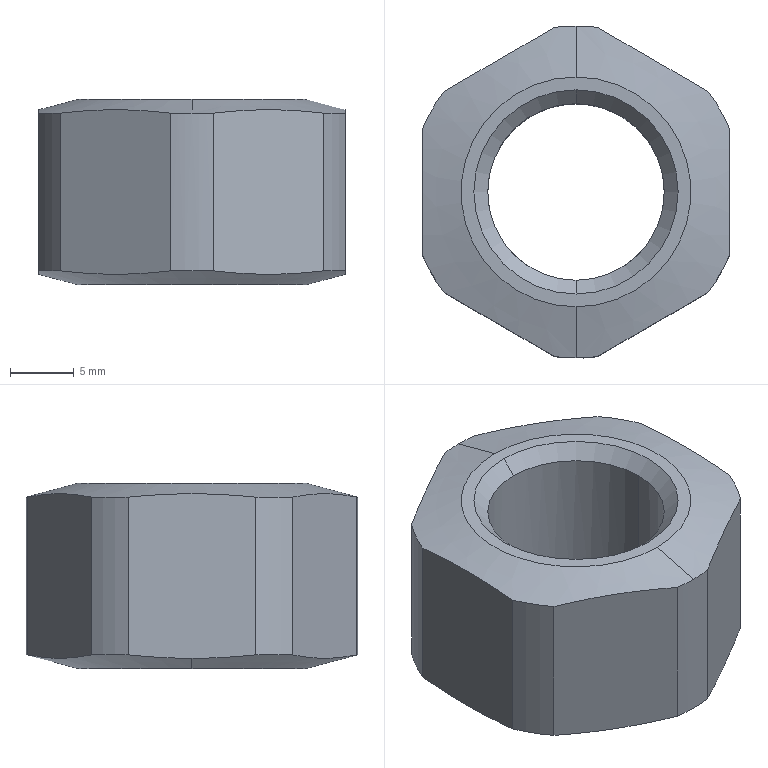Part | SolidWorks | features BaseBody 1 | 1 solid | 24 faces | box 24 x 26 x 14.5 mm | volume 4644 mm3 | cylinder 8 | cone 8 | plane 8 | commonest cylinder face diameters 26 x6 13.835 x2
STEP:
#1=CARTESIAN_POINT('',(-6.918,0.,-6.168));
#2=VERTEX_POINT('',#1);
#3=CARTESIAN_POINT('',(6.918,0.,-6.168));
#4=VERTEX_POINT('',#3);
#5=CARTESIAN_POINT('',(0.,0.,-6.168));
#6=DIRECTION('',(0.,0.,1.));
#7=DIRECTION('',(1.,0.,0.));
#8=AXIS2_PLACEMENT_3D('',#5,#6,#7);
#9=CIRCLE('',#8,6.918);
#10=EDGE_CURVE('',#2,#4,#9,.T.);
#11=ORIENTED_EDGE('',*,*,#10,.F.);
#12=CARTESIAN_POINT('',(-6.918,0.,6.168));
#13=VERTEX_POINT('',#12);
#14=CARTESIAN_POINT('',(-6.918,0.,-7.25));
#15=DIRECTION('',(0.,0.,1.));
#16=VECTOR('',#15,1000.);
#17=LINE('',#14,#16);
#18=EDGE_CURVE('',#2,#13,#17,.T.);
#19=ORIENTED_EDGE('',*,*,#18,.T.);
#20=CARTESIAN_POINT('',(0.,-6.918,6.168));
#21=VERTEX_POINT('',#20);
#22=CARTESIAN_POINT('',(0.,0.,6.168));
#23=DIRECTION('',(0.,0.,-1.));
#24=DIRECTION('',(1.,0.,0.));
#25=AXIS2_PLACEMENT_3D('',#22,#23,#24);
#26=CIRCLE('',#25,6.918);
#27=EDGE_CURVE('',#21,#13,#26,.T.);
#28=ORIENTED_EDGE('',*,*,#27,.F.);
#29=CARTESIAN_POINT('',(6.918,0.,6.168));
#30=VERTEX_POINT('',#29);
#31=CARTESIAN_POINT('',(0.,0.,6.168));
#32=DIRECTION('',(0.,0.,-1.));
#33=DIRECTION('',(1.,0.,0.));
#34=AXIS2_PLACEMENT_3D('',#31,#32,#33);
#35=CIRCLE('',#34,6.918);
#36=EDGE_CURVE('',#30,#21,#35,.T.);
#37=ORIENTED_EDGE('',*,*,#36,.F.);
#38=CARTESIAN_POINT('',(6.918,0.,-7.25));
#39=DIRECTION('',(0.,0.,1.));
#40=VECTOR('',#39,1000.);
#41=LINE('',#38,#40);
#42=EDGE_CURVE('',#4,#30,#41,.T.);
#43=ORIENTED_EDGE('',*,*,#42,.F.);
#44=EDGE_LOOP('',(#11,#19,#28,#37,#43));
#45=FACE_OUTER_BOUND('',#44,.T.);
#46=CARTESIAN_POINT('',(0.,0.,-7.25));
#47=DIRECTION('',(0.,0.,1.));
#48=DIRECTION('',(1.,0.,0.));
#49=AXIS2_PLACEMENT_3D('',#46,#47,#48);
#50=CYLINDRICAL_SURFACE('',#49,6.918);
#51=ADVANCED_FACE('',(#45),#50,.F.);
#52=ORIENTED_EDGE('',*,*,#27,.T.);
#53=CARTESIAN_POINT('',(0.,6.918,6.168));
#54=VERTEX_POINT('',#53);
#55=CARTESIAN_POINT('',(0.,0.,6.168));
#56=DIRECTION('',(0.,0.,-1.));
#57=DIRECTION('',(1.,0.,0.));
#58=AXIS2_PLACEMENT_3D('',#55,#56,#57);
#59=CIRCLE('',#58,6.918);
#60=EDGE_CURVE('',#13,#54,#59,.T.);
#61=ORIENTED_EDGE('',*,*,#60,.T.);
#62=CARTESIAN_POINT('',(0.,8.,7.25));
#63=VERTEX_POINT('',#62);
#64=CARTESIAN_POINT('',(0.,8.,7.25));
#65=DIRECTION('',(0.,0.7071,0.7071));
#66=VECTOR('',#65,1000.);
#67=LINE('',#64,#66);
#68=EDGE_CURVE('',#54,#63,#67,.T.);
#69=ORIENTED_EDGE('',*,*,#68,.T.);
#70=CARTESIAN_POINT('',(0.,-8.,7.25));
#71=VERTEX_POINT('',#70);
#72=CARTESIAN_POINT('',(0.,0.,7.25));
#73=DIRECTION('',(0.,0.,-1.));
#74=DIRECTION('',(0.,-1.,0.));
#75=AXIS2_PLACEMENT_3D('',#72,#73,#74);
#76=CIRCLE('',#75,8.);
#77=EDGE_CURVE('',#71,#63,#76,.T.);
#78=ORIENTED_EDGE('',*,*,#77,.F.);
#79=CARTESIAN_POINT('',(0.,-8.,7.25));
#80=DIRECTION('',(0.,-0.7071,0.7071));
#81=VECTOR('',#80,1000.);
#82=LINE('',#79,#81);
#83=EDGE_CURVE('',#21,#71,#82,.T.);
#84=ORIENTED_EDGE('',*,*,#83,.F.);
#85=EDGE_LOOP('',(#52,#61,#69,#78,#84));
#86=FACE_OUTER_BOUND('',#85,.T.);
#87=CARTESIAN_POINT('',(0.,0.,7.25));
#88=DIRECTION('',(0.,0.,1.));
#89=DIRECTION('',(0.,-1.,0.));
#90=AXIS2_PLACEMENT_3D('',#87,#88,#89);
#91=CONICAL_SURFACE('',#90,8.,0.7854);
#92=ADVANCED_FACE('',(#86),#91,.F.);
#93=ORIENTED_EDGE('',*,*,#10,.T.);
#94=CARTESIAN_POINT('',(8.,0.,-7.25));
#95=VERTEX_POINT('',#94);
#96=CARTESIAN_POINT('',(8.,0.,-7.25));
#97=DIRECTION('',(0.7071,0.,-0.7071));
#98=VECTOR('',#97,1000.);
#99=LINE('',#96,#98);
#100=EDGE_CURVE('',#4,#95,#99,.T.);
#101=ORIENTED_EDGE('',*,*,#100,.T.);
#102=CARTESIAN_POINT('',(-8.,0.,-7.25));
#103=VERTEX_POINT('',#102);
#104=CARTESIAN_POINT('',(0.,0.,-7.25));
#105=DIRECTION('',(0.,0.,1.));
#106=DIRECTION('',(-1.,0.,0.));
#107=AXIS2_PLACEMENT_3D('',#104,#105,#106);
#108=CIRCLE('',#107,8.);
#109=EDGE_CURVE('',#103,#95,#108,.T.);
#110=ORIENTED_EDGE('',*,*,#109,.F.);
#111=CARTESIAN_POINT('',(-8.,0.,-7.25));
#112=DIRECTION('',(-0.7071,0.,-0.7071));
#113=VECTOR('',#112,1000.);
#114=LINE('',#111,#113);
#115=EDGE_CURVE('',#2,#103,#114,.T.);
#116=ORIENTED_EDGE('',*,*,#115,.F.);
#117=EDGE_LOOP('',(#93,#101,#110,#116));
#118=FACE_OUTER_BOUND('',#117,.T.);
#119=CARTESIAN_POINT('',(0.,0.,-7.25));
#120=DIRECTION('',(0.,0.,-1.));
#121=DIRECTION('',(-1.,0.,0.));
#122=AXIS2_PLACEMENT_3D('',#119,#120,#121);
#123=CONICAL_SURFACE('',#122,8.,0.7854);
#124=ADVANCED_FACE('',(#118),#123,.F.);
#125=CARTESIAN_POINT('',(0.,9.,7.25));
#126=VERTEX_POINT('',#125);
#127=CARTESIAN_POINT('',(0.,-9.,7.25));
#128=VERTEX_POINT('',#127);
#129=CARTESIAN_POINT('',(0.,0.,7.25));
#130=DIRECTION('',(0.,0.,-1.));
#131=DIRECTION('',(0.,1.,0.));
#132=AXIS2_PLACEMENT_3D('',#129,#130,#131);
#133=CIRCLE('',#132,9.);
#134=EDGE_CURVE('',#126,#128,#133,.T.);
#135=ORIENTED_EDGE('',*,*,#134,.T.);
#136=CARTESIAN_POINT('',(0.,-13.,6.178));
#137=VERTEX_POINT('',#136);
#138=CARTESIAN_POINT('',(0.,-13.,6.178));
#139=DIRECTION('',(0.,-0.9659,-0.2588));
#140=VECTOR('',#139,1000.);
#141=LINE('',#138,#140);
#142=EDGE_CURVE('',#128,#137,#141,.T.);
#143=ORIENTED_EDGE('',*,*,#142,.T.);
#144=CARTESIAN_POINT('',(1.67,-12.892,6.178));
#145=VERTEX_POINT('',#144);
#146=CARTESIAN_POINT('',(0.,0.,6.178));
#147=DIRECTION('',(0.,0.,1.));
#148=DIRECTION('',(-1.,0.,0.));
#149=AXIS2_PLACEMENT_3D('',#146,#147,#148);
#150=CIRCLE('',#149,13.);
#151=EDGE_CURVE('',#137,#145,#150,.T.);
#152=ORIENTED_EDGE('',*,*,#151,.T.);
#153=CARTESIAN_POINT('',(10.33,-7.892,6.178));
#154=VERTEX_POINT('',#153);
#155=CARTESIAN_POINT('',(1.67,-12.892,6.178));
#156=CARTESIAN_POINT('',(3.113,-12.059,6.35));
#157=CARTESIAN_POINT('',(6.,-10.392,6.542));
#158=CARTESIAN_POINT('',(8.887,-8.726,6.35));
#159=CARTESIAN_POINT('',(10.33,-7.892,6.178));
#160=B_SPLINE_CURVE_WITH_KNOTS('',3,(#155,#156,#157,#158,#159),.UNSPECIFIED.,.F.,.F.,(4,1,4),(0.,0.005,0.01),.UNSPECIFIED.);
#161=EDGE_CURVE('',#145,#154,#160,.T.);
#162=ORIENTED_EDGE('',*,*,#161,.T.);
#163=CARTESIAN_POINT('',(12.,-5.,6.178));
#164=VERTEX_POINT('',#163);
#165=CARTESIAN_POINT('',(0.,0.,6.178));
#166=DIRECTION('',(0.,0.,1.));
#167=DIRECTION('',(-1.,0.,0.));
#168=AXIS2_PLACEMENT_3D('',#165,#166,#167);
#169=CIRCLE('',#168,13.);
#170=EDGE_CURVE('',#154,#164,#169,.T.);
#171=ORIENTED_EDGE('',*,*,#170,.T.);
#172=CARTESIAN_POINT('',(12.,5.,6.178));
#173=VERTEX_POINT('',#172);
#174=CARTESIAN_POINT('',(12.,-5.,6.178));
#175=CARTESIAN_POINT('',(12.,-3.333,6.35));
#176=CARTESIAN_POINT('',(12.,0.,6.542));
#177=CARTESIAN_POINT('',(12.,3.333,6.35));
#178=CARTESIAN_POINT('',(12.,5.,6.178));
#179=B_SPLINE_CURVE_WITH_KNOTS('',3,(#174,#175,#176,#177,#178),.UNSPECIFIED.,.F.,.F.,(4,1,4),(0.,0.005,0.01),.UNSPECIFIED.);
#180=EDGE_CURVE('',#164,#173,#179,.T.);
#181=ORIENTED_EDGE('',*,*,#180,.T.);
#182=CARTESIAN_POINT('',(10.33,7.892,6.178));
#183=VERTEX_POINT('',#182);
#184=CARTESIAN_POINT('',(0.,0.,6.178));
#185=DIRECTION('',(0.,0.,1.));
#186=DIRECTION('',(-1.,0.,0.));
#187=AXIS2_PLACEMENT_3D('',#184,#185,#186);
#188=CIRCLE('',#187,13.);
#189=EDGE_CURVE('',#173,#183,#188,.T.);
#190=ORIENTED_EDGE('',*,*,#189,.T.);
#191=CARTESIAN_POINT('',(1.67,12.892,6.178));
#192=VERTEX_POINT('',#191);
#193=CARTESIAN_POINT('',(10.33,7.892,6.178));
#194=CARTESIAN_POINT('',(8.887,8.726,6.35));
#195=CARTESIAN_POINT('',(6.,10.392,6.542));
#196=CARTESIAN_POINT('',(3.113,12.059,6.35));
#197=CARTESIAN_POINT('',(1.67,12.892,6.178));
#198=B_SPLINE_CURVE_WITH_KNOTS('',3,(#193,#194,#195,#196,#197),.UNSPECIFIED.,.F.,.F.,(4,1,4),(0.,0.005,0.01),.UNSPECIFIED.);
#199=EDGE_CURVE('',#183,#192,#198,.T.);
#200=ORIENTED_EDGE('',*,*,#199,.T.);
#201=CARTESIAN_POINT('',(0.,13.,6.178));
#202=VERTEX_POINT('',#201);
#203=CARTESIAN_POINT('',(0.,0.,6.178));
#204=DIRECTION('',(0.,0.,1.));
#205=DIRECTION('',(-1.,0.,0.));
#206=AXIS2_PLACEMENT_3D('',#203,#204,#205);
#207=CIRCLE('',#206,13.);
#208=EDGE_CURVE('',#192,#202,#207,.T.);
#209=ORIENTED_EDGE('',*,*,#208,.T.);
#210=CARTESIAN_POINT('',(0.,13.,6.178));
#211=DIRECTION('',(0.,0.9659,-0.2588));
#212=VECTOR('',#211,1000.);
#213=LINE('',#210,#212);
#214=EDGE_CURVE('',#126,#202,#213,.T.);
#215=ORIENTED_EDGE('',*,*,#214,.F.);
#216=EDGE_LOOP('',(#135,#143,#152,#162,#171,#181,#190,#200,#209,#215));
#217=FACE_OUTER_BOUND('',#216,.T.);
#218=CARTESIAN_POINT('',(0.,0.,6.178));
#219=DIRECTION('',(0.,0.,-1.));
#220=DIRECTION('',(0.,1.,0.));
#221=AXIS2_PLACEMENT_3D('',#218,#219,#220);
#222=CONICAL_SURFACE('',#221,13.,1.309);
#223=ADVANCED_FACE('',(#217),#222,.T.);
#224=CARTESIAN_POINT('',(9.,0.,-7.25));
#225=VERTEX_POINT('',#224);
#226=CARTESIAN_POINT('',(-9.,0.,-7.25));
#227=VERTEX_POINT('',#226);
#228=CARTESIAN_POINT('',(0.,0.,-7.25));
#229=DIRECTION('',(0.,0.,1.));
#230=DIRECTION('',(1.,0.,0.));
#231=AXIS2_PLACEMENT_3D('',#228,#229,#230);
#232=CIRCLE('',#231,9.);
#233=EDGE_CURVE('',#225,#227,#232,.T.);
#234=ORIENTED_EDGE('',*,*,#233,.T.);
#235=CARTESIAN_POINT('',(-12.,0.,-6.446));
#236=VERTEX_POINT('',#235);
#237=CARTESIAN_POINT('',(-13.,0.,-6.178));
#238=DIRECTION('',(-0.9659,0.,0.2588));
#239=VECTOR('',#238,1000.);
#240=LINE('',#237,#239);
#241=EDGE_CURVE('',#227,#236,#240,.T.);
#242=ORIENTED_EDGE('',*,*,#241,.T.);
#243=CARTESIAN_POINT('',(-12.,5.,-6.178));
#244=VERTEX_POINT('',#243);
#245=CARTESIAN_POINT('',(-12.,0.,-6.446));
#246=CARTESIAN_POINT('',(-12.,1.667,-6.446));
#247=CARTESIAN_POINT('',(-12.,3.333,-6.35));
#248=CARTESIAN_POINT('',(-12.,5.,-6.178));
#249=B_SPLINE_CURVE_WITH_KNOTS('',3,(#245,#246,#247,#248),.UNSPECIFIED.,.F.,.F.,(4,4),(0.005,0.01),.UNSPECIFIED.);
#250=EDGE_CURVE('',#236,#244,#249,.T.);
#251=ORIENTED_EDGE('',*,*,#250,.T.);
#252=CARTESIAN_POINT('',(-10.33,7.892,-6.178));
#253=VERTEX_POINT('',#252);
#254=CARTESIAN_POINT('',(0.,0.,-6.178));
#255=DIRECTION('',(0.,0.,-1.));
#256=DIRECTION('',(1.,0.,0.));
#257=AXIS2_PLACEMENT_3D('',#254,#255,#256);
#258=CIRCLE('',#257,13.);
#259=EDGE_CURVE('',#244,#253,#258,.T.);
#260=ORIENTED_EDGE('',*,*,#259,.T.);
#261=CARTESIAN_POINT('',(-1.67,12.892,-6.178));
#262=VERTEX_POINT('',#261);
#263=CARTESIAN_POINT('',(-10.33,7.892,-6.178));
#264=CARTESIAN_POINT('',(-8.887,8.726,-6.35));
#265=CARTESIAN_POINT('',(-6.,10.392,-6.542));
#266=CARTESIAN_POINT('',(-3.113,12.059,-6.35));
#267=CARTESIAN_POINT('',(-1.67,12.892,-6.178));
#268=B_SPLINE_CURVE_WITH_KNOTS('',3,(#263,#264,#265,#266,#267),.UNSPECIFIED.,.F.,.F.,(4,1,4),(0.,0.005,0.01),.UNSPECIFIED.);
#269=EDGE_CURVE('',#253,#262,#268,.T.);
#270=ORIENTED_EDGE('',*,*,#269,.T.);
#271=CARTESIAN_POINT('',(1.67,12.892,-6.178));
#272=VERTEX_POINT('',#271);
#273=CARTESIAN_POINT('',(0.,0.,-6.178));
#274=DIRECTION('',(0.,0.,-1.));
#275=DIRECTION('',(1.,0.,0.));
#276=AXIS2_PLACEMENT_3D('',#273,#274,#275);
#277=CIRCLE('',#276,13.);
#278=EDGE_CURVE('',#262,#272,#277,.T.);
#279=ORIENTED_EDGE('',*,*,#278,.T.);
#280=CARTESIAN_POINT('',(10.33,7.892,-6.178));
#281=VERTEX_POINT('',#280);
#282=CARTESIAN_POINT('',(1.67,12.892,-6.178));
#283=CARTESIAN_POINT('',(3.113,12.059,-6.35));
#284=CARTESIAN_POINT('',(6.,10.392,-6.542));
#285=CARTESIAN_POINT('',(8.887,8.726,-6.35));
#286=CARTESIAN_POINT('',(10.33,7.892,-6.178));
#287=B_SPLINE_CURVE_WITH_KNOTS('',3,(#282,#283,#284,#285,#286),.UNSPECIFIED.,.F.,.F.,(4,1,4),(0.,0.005,0.01),.UNSPECIFIED.);
#288=EDGE_CURVE('',#272,#281,#287,.T.);
#289=ORIENTED_EDGE('',*,*,#288,.T.);
#290=CARTESIAN_POINT('',(12.,5.,-6.178));
#291=VERTEX_POINT('',#290);
#292=CARTESIAN_POINT('',(0.,0.,-6.178));
#293=DIRECTION('',(0.,0.,-1.));
#294=DIRECTION('',(1.,0.,0.));
#295=AXIS2_PLACEMENT_3D('',#292,#293,#294);
#296=CIRCLE('',#295,13.);
#297=EDGE_CURVE('',#281,#291,#296,.T.);
#298=ORIENTED_EDGE('',*,*,#297,.T.);
#299=CARTESIAN_POINT('',(12.,0.,-6.446));
#300=VERTEX_POINT('',#299);
#301=CARTESIAN_POINT('',(12.,5.,-6.178));
#302=CARTESIAN_POINT('',(12.,3.333,-6.35));
#303=CARTESIAN_POINT('',(12.,1.667,-6.446));
#304=CARTESIAN_POINT('',(12.,0.,-6.446));
#305=B_SPLINE_CURVE_WITH_KNOTS('',3,(#301,#302,#303,#304),.UNSPECIFIED.,.F.,.F.,(4,4),(0.,0.005),.UNSPECIFIED.);
#306=EDGE_CURVE('',#291,#300,#305,.T.);
#307=ORIENTED_EDGE('',*,*,#306,.T.);
#308=CARTESIAN_POINT('',(13.,0.,-6.178));
#309=DIRECTION('',(0.9659,0.,0.2588));
#310=VECTOR('',#309,1000.);
#311=LINE('',#308,#310);
#312=EDGE_CURVE('',#225,#300,#311,.T.);
#313=ORIENTED_EDGE('',*,*,#312,.F.);
#314=EDGE_LOOP('',(#234,#242,#251,#260,#270,#279,#289,#298,#307,#313));
#315=FACE_OUTER_BOUND('',#314,.T.);
#316=CARTESIAN_POINT('',(0.,0.,-6.178));
#317=DIRECTION('',(0.,0.,1.));
#318=DIRECTION('',(1.,0.,0.));
#319=AXIS2_PLACEMENT_3D('',#316,#317,#318);
#320=CONICAL_SURFACE('',#319,13.,1.309);
#321=ADVANCED_FACE('',(#315),#320,.T.);
#322=ORIENTED_EDGE('',*,*,#18,.F.);
#323=CARTESIAN_POINT('',(0.,0.,-6.168));
#324=DIRECTION('',(0.,0.,1.));
#325=DIRECTION('',(1.,0.,0.));
#326=AXIS2_PLACEMENT_3D('',#323,#324,#325);
#327=CIRCLE('',#326,6.918);
#328=EDGE_CURVE('',#4,#2,#327,.T.);
#329=ORIENTED_EDGE('',*,*,#328,.F.);
#330=ORIENTED_EDGE('',*,*,#42,.T.);
#331=CARTESIAN_POINT('',(0.,0.,6.168));
#332=DIRECTION('',(0.,0.,-1.));
#333=DIRECTION('',(1.,0.,0.));
#334=AXIS2_PLACEMENT_3D('',#331,#332,#333);
#335=CIRCLE('',#334,6.918);
#336=EDGE_CURVE('',#54,#30,#335,.T.);
#337=ORIENTED_EDGE('',*,*,#336,.F.);
#338=ORIENTED_EDGE('',*,*,#60,.F.);
#339=EDGE_LOOP('',(#322,#329,#330,#337,#338));
#340=FACE_OUTER_BOUND('',#339,.T.);
#341=CARTESIAN_POINT('',(0.,0.,-7.25));
#342=DIRECTION('',(0.,0.,1.));
#343=DIRECTION('',(1.,0.,0.));
#344=AXIS2_PLACEMENT_3D('',#341,#342,#343);
#345=CYLINDRICAL_SURFACE('',#344,6.918);
#346=ADVANCED_FACE('',(#340),#345,.F.);
#347=ORIENTED_EDGE('',*,*,#68,.F.);
#348=ORIENTED_EDGE('',*,*,#336,.T.);
#349=ORIENTED_EDGE('',*,*,#36,.T.);
#350=ORIENTED_EDGE('',*,*,#83,.T.);
#351=CARTESIAN_POINT('',(0.,0.,7.25));
#352=DIRECTION('',(0.,0.,-1.));
#353=DIRECTION('',(0.,-1.,0.));
#354=AXIS2_PLACEMENT_3D('',#351,#352,#353);
#355=CIRCLE('',#354,8.);
#356=EDGE_CURVE('',#63,#71,#355,.T.);
#357=ORIENTED_EDGE('',*,*,#356,.F.);
#358=EDGE_LOOP('',(#347,#348,#349,#350,#357));
#359=FACE_OUTER_BOUND('',#358,.T.);
#360=CARTESIAN_POINT('',(0.,0.,7.25));
#361=DIRECTION('',(0.,0.,1.));
#362=DIRECTION('',(0.,-1.,0.));
#363=AXIS2_PLACEMENT_3D('',#360,#361,#362);
#364=CONICAL_SURFACE('',#363,8.,0.7854);
#365=ADVANCED_FACE('',(#359),#364,.F.);
#366=ORIENTED_EDGE('',*,*,#100,.F.);
#367=ORIENTED_EDGE('',*,*,#328,.T.);
#368=ORIENTED_EDGE('',*,*,#115,.T.);
#369=CARTESIAN_POINT('',(0.,0.,-7.25));
#370=DIRECTION('',(0.,0.,1.));
#371=DIRECTION('',(-1.,0.,0.));
#372=AXIS2_PLACEMENT_3D('',#369,#370,#371);
#373=CIRCLE('',#372,8.);
#374=EDGE_CURVE('',#95,#103,#373,.T.);
#375=ORIENTED_EDGE('',*,*,#374,.F.);
#376=EDGE_LOOP('',(#366,#367,#368,#375));
#377=FACE_OUTER_BOUND('',#376,.T.);
#378=CARTESIAN_POINT('',(0.,0.,-7.25));
#379=DIRECTION('',(0.,0.,-1.));
#380=DIRECTION('',(-1.,0.,0.));
#381=AXIS2_PLACEMENT_3D('',#378,#379,#380);
#382=CONICAL_SURFACE('',#381,8.,0.7854);
#383=ADVANCED_FACE('',(#377),#382,.F.);
#384=ORIENTED_EDGE('',*,*,#77,.T.);
#385=ORIENTED_EDGE('',*,*,#356,.T.);
#386=EDGE_LOOP('',(#384,#385));
#387=FACE_BOUND('',#386,.T.);
#388=ORIENTED_EDGE('',*,*,#134,.F.);
#389=CARTESIAN_POINT('',(0.,0.,7.25));
#390=DIRECTION('',(0.,0.,-1.));
#391=DIRECTION('',(0.,1.,0.));
#392=AXIS2_PLACEMENT_3D('',#389,#390,#391);
#393=CIRCLE('',#392,9.);
#394=EDGE_CURVE('',#128,#126,#393,.T.);
#395=ORIENTED_EDGE('',*,*,#394,.F.);
#396=EDGE_LOOP('',(#388,#395));
#397=FACE_OUTER_BOUND('',#396,.T.);
#398=CARTESIAN_POINT('',(0.,0.,7.25));
#399=DIRECTION('',(0.,0.,-1.));
#400=DIRECTION('',(-1.,0.,0.));
#401=AXIS2_PLACEMENT_3D('',#398,#399,#400);
#402=PLANE('',#401);
#403=ADVANCED_FACE('',(#387,#397),#402,.F.);
#404=ORIENTED_EDGE('',*,*,#233,.F.);
#405=CARTESIAN_POINT('',(0.,0.,-7.25));
#406=DIRECTION('',(0.,0.,1.));
#407=DIRECTION('',(1.,0.,0.));
#408=AXIS2_PLACEMENT_3D('',#405,#406,#407);
#409=CIRCLE('',#408,9.);
#410=EDGE_CURVE('',#227,#225,#409,.T.);
#411=ORIENTED_EDGE('',*,*,#410,.F.);
#412=EDGE_LOOP('',(#404,#411));
#413=FACE_OUTER_BOUND('',#412,.T.);
#414=ORIENTED_EDGE('',*,*,#109,.T.);
#415=ORIENTED_EDGE('',*,*,#374,.T.);
#416=EDGE_LOOP('',(#414,#415));
#417=FACE_BOUND('',#416,.T.);
#418=CARTESIAN_POINT('',(0.,9.,-7.25));
#419=DIRECTION('',(0.,0.,1.));
#420=DIRECTION('',(1.,0.,0.));
#421=AXIS2_PLACEMENT_3D('',#418,#419,#420);
#422=PLANE('',#421);
#423=ADVANCED_FACE('',(#413,#417),#422,.F.);
#424=ORIENTED_EDGE('',*,*,#142,.F.);
#425=ORIENTED_EDGE('',*,*,#394,.T.);
#426=ORIENTED_EDGE('',*,*,#214,.T.);
#427=CARTESIAN_POINT('',(-1.67,12.892,6.178));
#428=VERTEX_POINT('',#427);
#429=CARTESIAN_POINT('',(0.,0.,6.178));
#430=DIRECTION('',(0.,0.,1.));
#431=DIRECTION('',(-1.,0.,0.));
#432=AXIS2_PLACEMENT_3D('',#429,#430,#431);
#433=CIRCLE('',#432,13.);
#434=EDGE_CURVE('',#202,#428,#433,.T.);
#435=ORIENTED_EDGE('',*,*,#434,.T.);
#436=CARTESIAN_POINT('',(-10.33,7.892,6.178));
#437=VERTEX_POINT('',#436);
#438=CARTESIAN_POINT('',(-1.67,12.892,6.178));
#439=CARTESIAN_POINT('',(-3.113,12.059,6.35));
#440=CARTESIAN_POINT('',(-6.,10.392,6.542));
#441=CARTESIAN_POINT('',(-8.887,8.726,6.35));
#442=CARTESIAN_POINT('',(-10.33,7.892,6.178));
#443=B_SPLINE_CURVE_WITH_KNOTS('',3,(#438,#439,#440,#441,#442),.UNSPECIFIED.,.F.,.F.,(4,1,4),(0.,0.005,0.01),.UNSPECIFIED.);
#444=EDGE_CURVE('',#428,#437,#443,.T.);
#445=ORIENTED_EDGE('',*,*,#444,.T.);
#446=CARTESIAN_POINT('',(-12.,5.,6.178));
#447=VERTEX_POINT('',#446);
#448=CARTESIAN_POINT('',(0.,0.,6.178));
#449=DIRECTION('',(0.,0.,1.));
#450=DIRECTION('',(-1.,0.,0.));
#451=AXIS2_PLACEMENT_3D('',#448,#449,#450);
#452=CIRCLE('',#451,13.);
#453=EDGE_CURVE('',#437,#447,#452,.T.);
#454=ORIENTED_EDGE('',*,*,#453,.T.);
#455=CARTESIAN_POINT('',(-12.,-5.,6.178));
#456=VERTEX_POINT('',#455);
#457=CARTESIAN_POINT('',(-12.,5.,6.178));
#458=CARTESIAN_POINT('',(-12.,3.333,6.35));
#459=CARTESIAN_POINT('',(-12.,0.,6.542));
#460=CARTESIAN_POINT('',(-12.,-3.333,6.35));
#461=CARTESIAN_POINT('',(-12.,-5.,6.178));
#462=B_SPLINE_CURVE_WITH_KNOTS('',3,(#457,#458,#459,#460,#461),.UNSPECIFIED.,.F.,.F.,(4,1,4),(0.,0.005,0.01),.UNSPECIFIED.);
#463=EDGE_CURVE('',#447,#456,#462,.T.);
#464=ORIENTED_EDGE('',*,*,#463,.T.);
#465=CARTESIAN_POINT('',(-10.33,-7.892,6.178));
#466=VERTEX_POINT('',#465);
#467=CARTESIAN_POINT('',(0.,0.,6.178));
#468=DIRECTION('',(0.,0.,1.));
#469=DIRECTION('',(-1.,0.,0.));
#470=AXIS2_PLACEMENT_3D('',#467,#468,#469);
#471=CIRCLE('',#470,13.);
#472=EDGE_CURVE('',#456,#466,#471,.T.);
#473=ORIENTED_EDGE('',*,*,#472,.T.);
#474=CARTESIAN_POINT('',(-1.67,-12.892,6.178));
#475=VERTEX_POINT('',#474);
#476=CARTESIAN_POINT('',(-10.33,-7.892,6.178));
#477=CARTESIAN_POINT('',(-8.887,-8.726,6.35));
#478=CARTESIAN_POINT('',(-6.,-10.392,6.542));
#479=CARTESIAN_POINT('',(-3.113,-12.059,6.35));
#480=CARTESIAN_POINT('',(-1.67,-12.892,6.178));
#481=B_SPLINE_CURVE_WITH_KNOTS('',3,(#476,#477,#478,#479,#480),.UNSPECIFIED.,.F.,.F.,(4,1,4),(0.,0.005,0.01),.UNSPECIFIED.);
#482=EDGE_CURVE('',#466,#475,#481,.T.);
#483=ORIENTED_EDGE('',*,*,#482,.T.);
#484=CARTESIAN_POINT('',(0.,0.,6.178));
#485=DIRECTION('',(0.,0.,1.));
#486=DIRECTION('',(-1.,0.,0.));
#487=AXIS2_PLACEMENT_3D('',#484,#485,#486);
#488=CIRCLE('',#487,13.);
#489=EDGE_CURVE('',#475,#137,#488,.T.);
#490=ORIENTED_EDGE('',*,*,#489,.T.);
#491=EDGE_LOOP('',(#424,#425,#426,#435,#445,#454,#464,#473,#483,#490));
#492=FACE_OUTER_BOUND('',#491,.T.);
#493=CARTESIAN_POINT('',(0.,0.,6.178));
#494=DIRECTION('',(0.,0.,-1.));
#495=DIRECTION('',(0.,1.,0.));
#496=AXIS2_PLACEMENT_3D('',#493,#494,#495);
#497=CONICAL_SURFACE('',#496,13.,1.309);
#498=ADVANCED_FACE('',(#492),#497,.T.);
#499=ORIENTED_EDGE('',*,*,#241,.F.);
#500=ORIENTED_EDGE('',*,*,#410,.T.);
#501=ORIENTED_EDGE('',*,*,#312,.T.);
#502=CARTESIAN_POINT('',(12.,-5.,-6.178));
#503=VERTEX_POINT('',#502);
#504=CARTESIAN_POINT('',(12.,0.,-6.446));
#505=CARTESIAN_POINT('',(12.,-1.667,-6.446));
#506=CARTESIAN_POINT('',(12.,-3.333,-6.35));
#507=CARTESIAN_POINT('',(12.,-5.,-6.178));
#508=B_SPLINE_CURVE_WITH_KNOTS('',3,(#504,#505,#506,#507),.UNSPECIFIED.,.F.,.F.,(4,4),(0.005,0.01),.UNSPECIFIED.);
#509=EDGE_CURVE('',#300,#503,#508,.T.);
#510=ORIENTED_EDGE('',*,*,#509,.T.);
#511=CARTESIAN_POINT('',(10.33,-7.892,-6.178));
#512=VERTEX_POINT('',#511);
#513=CARTESIAN_POINT('',(0.,0.,-6.178));
#514=DIRECTION('',(0.,0.,-1.));
#515=DIRECTION('',(1.,0.,0.));
#516=AXIS2_PLACEMENT_3D('',#513,#514,#515);
#517=CIRCLE('',#516,13.);
#518=EDGE_CURVE('',#503,#512,#517,.T.);
#519=ORIENTED_EDGE('',*,*,#518,.T.);
#520=CARTESIAN_POINT('',(1.67,-12.892,-6.178));
#521=VERTEX_POINT('',#520);
#522=CARTESIAN_POINT('',(10.33,-7.892,-6.178));
#523=CARTESIAN_POINT('',(8.887,-8.726,-6.35));
#524=CARTESIAN_POINT('',(6.,-10.392,-6.542));
#525=CARTESIAN_POINT('',(3.113,-12.059,-6.35));
#526=CARTESIAN_POINT('',(1.67,-12.892,-6.178));
#527=B_SPLINE_CURVE_WITH_KNOTS('',3,(#522,#523,#524,#525,#526),.UNSPECIFIED.,.F.,.F.,(4,1,4),(0.,0.005,0.01),.UNSPECIFIED.);
#528=EDGE_CURVE('',#512,#521,#527,.T.);
#529=ORIENTED_EDGE('',*,*,#528,.T.);
#530=CARTESIAN_POINT('',(-1.67,-12.892,-6.178));
#531=VERTEX_POINT('',#530);
#532=CARTESIAN_POINT('',(0.,0.,-6.178));
#533=DIRECTION('',(0.,0.,-1.));
#534=DIRECTION('',(1.,0.,0.));
#535=AXIS2_PLACEMENT_3D('',#532,#533,#534);
#536=CIRCLE('',#535,13.);
#537=EDGE_CURVE('',#521,#531,#536,.T.);
#538=ORIENTED_EDGE('',*,*,#537,.T.);
#539=CARTESIAN_POINT('',(-10.33,-7.892,-6.178));
#540=VERTEX_POINT('',#539);
#541=CARTESIAN_POINT('',(-1.67,-12.892,-6.178));
#542=CARTESIAN_POINT('',(-3.113,-12.059,-6.35));
#543=CARTESIAN_POINT('',(-6.,-10.392,-6.542));
#544=CARTESIAN_POINT('',(-8.887,-8.726,-6.35));
#545=CARTESIAN_POINT('',(-10.33,-7.892,-6.178));
#546=B_SPLINE_CURVE_WITH_KNOTS('',3,(#541,#542,#543,#544,#545),.UNSPECIFIED.,.F.,.F.,(4,1,4),(0.,0.005,0.01),.UNSPECIFIED.);
#547=EDGE_CURVE('',#531,#540,#546,.T.);
#548=ORIENTED_EDGE('',*,*,#547,.T.);
#549=CARTESIAN_POINT('',(-12.,-5.,-6.178));
#550=VERTEX_POINT('',#549);
#551=CARTESIAN_POINT('',(0.,0.,-6.178));
#552=DIRECTION('',(0.,0.,-1.));
#553=DIRECTION('',(1.,0.,0.));
#554=AXIS2_PLACEMENT_3D('',#551,#552,#553);
#555=CIRCLE('',#554,13.);
#556=EDGE_CURVE('',#540,#550,#555,.T.);
#557=ORIENTED_EDGE('',*,*,#556,.T.);
#558=CARTESIAN_POINT('',(-12.,-5.,-6.178));
#559=CARTESIAN_POINT('',(-12.,-3.333,-6.35));
#560=CARTESIAN_POINT('',(-12.,-1.667,-6.446));
#561=CARTESIAN_POINT('',(-12.,0.,-6.446));
#562=B_SPLINE_CURVE_WITH_KNOTS('',3,(#558,#559,#560,#561),.UNSPECIFIED.,.F.,.F.,(4,4),(0.,0.005),.UNSPECIFIED.);
#563=EDGE_CURVE('',#550,#236,#562,.T.);
#564=ORIENTED_EDGE('',*,*,#563,.T.);
#565=EDGE_LOOP('',(#499,#500,#501,#510,#519,#529,#538,#548,#557,#564));
#566=FACE_OUTER_BOUND('',#565,.T.);
#567=CARTESIAN_POINT('',(0.,0.,-6.178));
#568=DIRECTION('',(0.,0.,1.));
#569=DIRECTION('',(1.,0.,0.));
#570=AXIS2_PLACEMENT_3D('',#567,#568,#569);
#571=CONICAL_SURFACE('',#570,13.,1.309);
#572=ADVANCED_FACE('',(#566),#571,.T.);
#573=CARTESIAN_POINT('',(1.67,12.892,7.25));
#574=DIRECTION('',(0.,0.,-1.));
#575=VECTOR('',#574,1000.);
#576=LINE('',#573,#575);
#577=EDGE_CURVE('',#192,#272,#576,.T.);
#578=ORIENTED_EDGE('',*,*,#577,.F.);
#579=ORIENTED_EDGE('',*,*,#199,.F.);
#580=CARTESIAN_POINT('',(10.33,7.892,7.25));
#581=DIRECTION('',(0.,0.,1.));
#582=VECTOR('',#581,1000.);
#583=LINE('',#580,#582);
#584=EDGE_CURVE('',#281,#183,#583,.T.);
#585=ORIENTED_EDGE('',*,*,#584,.F.);
#586=ORIENTED_EDGE('',*,*,#288,.F.);
#587=EDGE_LOOP('',(#578,#579,#585,#586));
#588=FACE_OUTER_BOUND('',#587,.T.);
#589=CARTESIAN_POINT('',(12.,6.928,7.25));
#590=DIRECTION('',(-0.5,-0.866,0.));
#591=DIRECTION('',(0.866,-0.5,0.));
#592=AXIS2_PLACEMENT_3D('',#589,#590,#591);
#593=PLANE('',#592);
#594=ADVANCED_FACE('',(#588),#593,.F.);
#595=ORIENTED_EDGE('',*,*,#584,.T.);
#596=ORIENTED_EDGE('',*,*,#189,.F.);
#597=CARTESIAN_POINT('',(12.,5.,7.25));
#598=DIRECTION('',(0.,0.,-1.));
#599=VECTOR('',#598,1000.);
#600=LINE('',#597,#599);
#601=EDGE_CURVE('',#173,#291,#600,.T.);
#602=ORIENTED_EDGE('',*,*,#601,.T.);
#603=ORIENTED_EDGE('',*,*,#297,.F.);
#604=EDGE_LOOP('',(#595,#596,#602,#603));
#605=FACE_OUTER_BOUND('',#604,.T.);
#606=CARTESIAN_POINT('',(0.,0.,7.25));
#607=DIRECTION('',(0.,0.,1.));
#608=DIRECTION('',(1.,0.,0.));
#609=AXIS2_PLACEMENT_3D('',#606,#607,#608);
#610=CYLINDRICAL_SURFACE('',#609,13.);
#611=ADVANCED_FACE('',(#605),#610,.T.);
#612=ORIENTED_EDGE('',*,*,#601,.F.);
#613=ORIENTED_EDGE('',*,*,#180,.F.);
#614=CARTESIAN_POINT('',(12.,-5.,7.25));
#615=DIRECTION('',(0.,0.,1.));
#616=VECTOR('',#615,1000.);
#617=LINE('',#614,#616);
#618=EDGE_CURVE('',#503,#164,#617,.T.);
#619=ORIENTED_EDGE('',*,*,#618,.F.);
#620=ORIENTED_EDGE('',*,*,#509,.F.);
#621=ORIENTED_EDGE('',*,*,#306,.F.);
#622=EDGE_LOOP('',(#612,#613,#619,#620,#621));
#623=FACE_OUTER_BOUND('',#622,.T.);
#624=CARTESIAN_POINT('',(12.,-6.928,7.25));
#625=DIRECTION('',(-1.,0.,0.));
#626=DIRECTION('',(0.,0.,1.));
#627=AXIS2_PLACEMENT_3D('',#624,#625,#626);
#628=PLANE('',#627);
#629=ADVANCED_FACE('',(#623),#628,.F.);
#630=ORIENTED_EDGE('',*,*,#618,.T.);
#631=ORIENTED_EDGE('',*,*,#170,.F.);
#632=CARTESIAN_POINT('',(10.33,-7.892,7.25));
#633=DIRECTION('',(0.,0.,-1.));
#634=VECTOR('',#633,1000.);
#635=LINE('',#632,#634);
#636=EDGE_CURVE('',#154,#512,#635,.T.);
#637=ORIENTED_EDGE('',*,*,#636,.T.);
#638=ORIENTED_EDGE('',*,*,#518,.F.);
#639=EDGE_LOOP('',(#630,#631,#637,#638));
#640=FACE_OUTER_BOUND('',#639,.T.);
#641=CARTESIAN_POINT('',(0.,0.,7.25));
#642=DIRECTION('',(0.,0.,1.));
#643=DIRECTION('',(1.,0.,0.));
#644=AXIS2_PLACEMENT_3D('',#641,#642,#643);
#645=CYLINDRICAL_SURFACE('',#644,13.);
#646=ADVANCED_FACE('',(#640),#645,.T.);
#647=ORIENTED_EDGE('',*,*,#636,.F.);
#648=ORIENTED_EDGE('',*,*,#161,.F.);
#649=CARTESIAN_POINT('',(1.67,-12.892,7.25));
#650=DIRECTION('',(0.,0.,1.));
#651=VECTOR('',#650,1000.);
#652=LINE('',#649,#651);
#653=EDGE_CURVE('',#521,#145,#652,.T.);
#654=ORIENTED_EDGE('',*,*,#653,.F.);
#655=ORIENTED_EDGE('',*,*,#528,.F.);
#656=EDGE_LOOP('',(#647,#648,#654,#655));
#657=FACE_OUTER_BOUND('',#656,.T.);
#658=CARTESIAN_POINT('',(0.,-13.856,7.25));
#659=DIRECTION('',(-0.5,0.866,0.));
#660=DIRECTION('',(-0.866,-0.5,0.));
#661=AXIS2_PLACEMENT_3D('',#658,#659,#660);
#662=PLANE('',#661);
#663=ADVANCED_FACE('',(#657),#662,.F.);
#664=ORIENTED_EDGE('',*,*,#653,.T.);
#665=ORIENTED_EDGE('',*,*,#151,.F.);
#666=ORIENTED_EDGE('',*,*,#489,.F.);
#667=CARTESIAN_POINT('',(-1.67,-12.892,7.25));
#668=DIRECTION('',(0.,0.,-1.));
#669=VECTOR('',#668,1000.);
#670=LINE('',#667,#669);
#671=EDGE_CURVE('',#475,#531,#670,.T.);
#672=ORIENTED_EDGE('',*,*,#671,.T.);
#673=ORIENTED_EDGE('',*,*,#537,.F.);
#674=EDGE_LOOP('',(#664,#665,#666,#672,#673));
#675=FACE_OUTER_BOUND('',#674,.T.);
#676=CARTESIAN_POINT('',(0.,0.,7.25));
#677=DIRECTION('',(0.,0.,1.));
#678=DIRECTION('',(1.,0.,0.));
#679=AXIS2_PLACEMENT_3D('',#676,#677,#678);
#680=CYLINDRICAL_SURFACE('',#679,13.);
#681=ADVANCED_FACE('',(#675),#680,.T.);
#682=ORIENTED_EDGE('',*,*,#671,.F.);
#683=ORIENTED_EDGE('',*,*,#482,.F.);
#684=CARTESIAN_POINT('',(-10.33,-7.892,7.25));
#685=DIRECTION('',(0.,0.,1.));
#686=VECTOR('',#685,1000.);
#687=LINE('',#684,#686);
#688=EDGE_CURVE('',#540,#466,#687,.T.);
#689=ORIENTED_EDGE('',*,*,#688,.F.);
#690=ORIENTED_EDGE('',*,*,#547,.F.);
#691=EDGE_LOOP('',(#682,#683,#689,#690));
#692=FACE_OUTER_BOUND('',#691,.T.);
#693=CARTESIAN_POINT('',(-12.,-6.928,7.25));
#694=DIRECTION('',(0.5,0.866,0.));
#695=DIRECTION('',(-0.866,0.5,0.));
#696=AXIS2_PLACEMENT_3D('',#693,#694,#695);
#697=PLANE('',#696);
#698=ADVANCED_FACE('',(#692),#697,.F.);
#699=ORIENTED_EDGE('',*,*,#688,.T.);
#700=ORIENTED_EDGE('',*,*,#472,.F.);
#701=CARTESIAN_POINT('',(-12.,-5.,7.25));
#702=DIRECTION('',(0.,0.,-1.));
#703=VECTOR('',#702,1000.);
#704=LINE('',#701,#703);
#705=EDGE_CURVE('',#456,#550,#704,.T.);
#706=ORIENTED_EDGE('',*,*,#705,.T.);
#707=ORIENTED_EDGE('',*,*,#556,.F.);
#708=EDGE_LOOP('',(#699,#700,#706,#707));
#709=FACE_OUTER_BOUND('',#708,.T.);
#710=CARTESIAN_POINT('',(0.,0.,7.25));
#711=DIRECTION('',(0.,0.,1.));
#712=DIRECTION('',(1.,0.,0.));
#713=AXIS2_PLACEMENT_3D('',#710,#711,#712);
#714=CYLINDRICAL_SURFACE('',#713,13.);
#715=ADVANCED_FACE('',(#709),#714,.T.);
#716=ORIENTED_EDGE('',*,*,#705,.F.);
#717=ORIENTED_EDGE('',*,*,#463,.F.);
#718=CARTESIAN_POINT('',(-12.,5.,7.25));
#719=DIRECTION('',(0.,0.,1.));
#720=VECTOR('',#719,1000.);
#721=LINE('',#718,#720);
#722=EDGE_CURVE('',#244,#447,#721,.T.);
#723=ORIENTED_EDGE('',*,*,#722,.F.);
#724=ORIENTED_EDGE('',*,*,#250,.F.);
#725=ORIENTED_EDGE('',*,*,#563,.F.);
#726=EDGE_LOOP('',(#716,#717,#723,#724,#725));
#727=FACE_OUTER_BOUND('',#726,.T.);
#728=CARTESIAN_POINT('',(-12.,6.928,7.25));
#729=DIRECTION('',(1.,0.,0.));
#730=DIRECTION('',(0.,0.,-1.));
#731=AXIS2_PLACEMENT_3D('',#728,#729,#730);
#732=PLANE('',#731);
#733=ADVANCED_FACE('',(#727),#732,.F.);
#734=ORIENTED_EDGE('',*,*,#722,.T.);
#735=ORIENTED_EDGE('',*,*,#453,.F.);
#736=CARTESIAN_POINT('',(-10.33,7.892,7.25));
#737=DIRECTION('',(0.,0.,-1.));
#738=VECTOR('',#737,1000.);
#739=LINE('',#736,#738);
#740=EDGE_CURVE('',#437,#253,#739,.T.);
#741=ORIENTED_EDGE('',*,*,#740,.T.);
#742=ORIENTED_EDGE('',*,*,#259,.F.);
#743=EDGE_LOOP('',(#734,#735,#741,#742));
#744=FACE_OUTER_BOUND('',#743,.T.);
#745=CARTESIAN_POINT('',(0.,0.,7.25));
#746=DIRECTION('',(0.,0.,1.));
#747=DIRECTION('',(1.,0.,0.));
#748=AXIS2_PLACEMENT_3D('',#745,#746,#747);
#749=CYLINDRICAL_SURFACE('',#748,13.);
#750=ADVANCED_FACE('',(#744),#749,.T.);
#751=ORIENTED_EDGE('',*,*,#740,.F.);
#752=ORIENTED_EDGE('',*,*,#444,.F.);
#753=CARTESIAN_POINT('',(-1.67,12.892,7.25));
#754=DIRECTION('',(0.,0.,1.));
#755=VECTOR('',#754,1000.);
#756=LINE('',#753,#755);
#757=EDGE_CURVE('',#262,#428,#756,.T.);
#758=ORIENTED_EDGE('',*,*,#757,.F.);
#759=ORIENTED_EDGE('',*,*,#269,.F.);
#760=EDGE_LOOP('',(#751,#752,#758,#759));
#761=FACE_OUTER_BOUND('',#760,.T.);
#762=CARTESIAN_POINT('',(0.,13.856,7.25));
#763=DIRECTION('',(0.5,-0.866,0.));
#764=DIRECTION('',(0.866,0.5,0.));
#765=AXIS2_PLACEMENT_3D('',#762,#763,#764);
#766=PLANE('',#765);
#767=ADVANCED_FACE('',(#761),#766,.F.);
#768=ORIENTED_EDGE('',*,*,#757,.T.);
#769=ORIENTED_EDGE('',*,*,#434,.F.);
#770=ORIENTED_EDGE('',*,*,#208,.F.);
#771=ORIENTED_EDGE('',*,*,#577,.T.);
#772=ORIENTED_EDGE('',*,*,#278,.F.);
#773=EDGE_LOOP('',(#768,#769,#770,#771,#772));
#774=FACE_OUTER_BOUND('',#773,.T.);
#775=CARTESIAN_POINT('',(0.,0.,7.25));
#776=DIRECTION('',(0.,0.,1.));
#777=DIRECTION('',(1.,0.,0.));
#778=AXIS2_PLACEMENT_3D('',#775,#776,#777);
#779=CYLINDRICAL_SURFACE('',#778,13.);
#780=ADVANCED_FACE('',(#774),#779,.T.);
#781=CLOSED_SHELL('',(#51,#92,#124,#223,#321,#346,#365,#383,#403,#423,#498,#572,#594,#611,#629,#646,#663,#681,#698,#715,#733,#750,#767,#780));
#782=MANIFOLD_SOLID_BREP('',#781);
#783=CARTESIAN_POINT('',(0.,0.,0.));
#784=DIRECTION('',(0.,0.,1.));
#785=DIRECTION('',(1.,0.,0.));
#786=AXIS2_PLACEMENT_3D('',#783,#784,#785);
#787=(LENGTH_UNIT()NAMED_UNIT(*)SI_UNIT(.MILLI.,.METRE.));
#788=UNCERTAINTY_MEASURE_WITH_UNIT(LENGTH_MEASURE(0.00001),#787,'','');
#789=(NAMED_UNIT(*)PLANE_ANGLE_UNIT()SI_UNIT($,.RADIAN.));
#790=(NAMED_UNIT(*)SI_UNIT($,.STERADIAN.)SOLID_ANGLE_UNIT());
#791=(GEOMETRIC_REPRESENTATION_CONTEXT(3)GLOBAL_UNCERTAINTY_ASSIGNED_CONTEXT((#788))GLOBAL_UNIT_ASSIGNED_CONTEXT((#787,#789,#790))REPRESENTATION_CONTEXT('',''));
#792=ADVANCED_BREP_SHAPE_REPRESENTATION('',(#782,#786),#791);